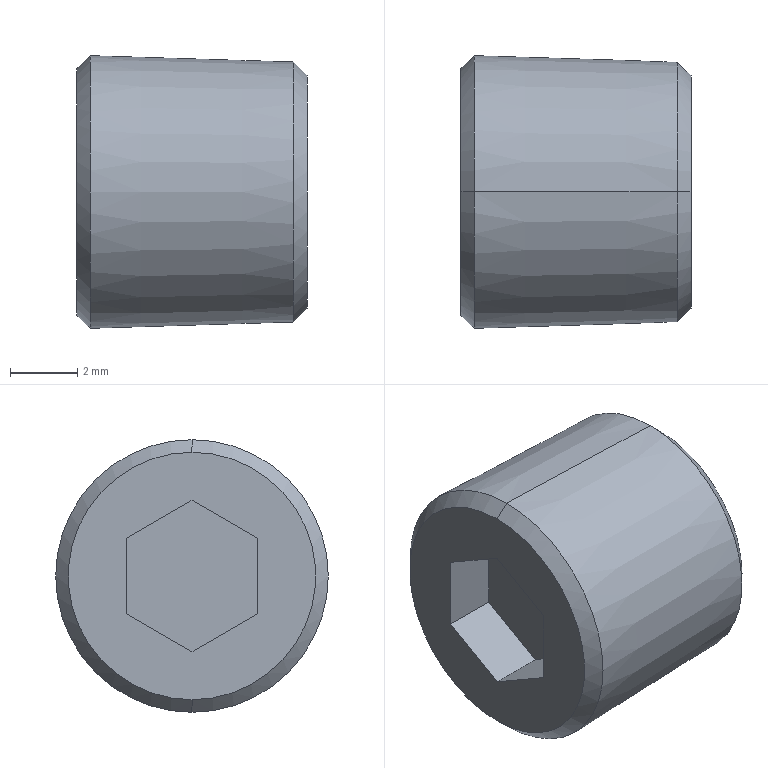Part | STEP file | AC10B-M5_AC3011A Plug(00) | 1 solid | 15 faces | box 6.85 x 8.115 x 8.115 mm | volume 313.171 mm3 | plane 9 | cone 6
STEP:
#1=CARTESIAN_POINT('',(0.,0.,0.));
#2=DIRECTION('',(0.,0.,1.));
#3=DIRECTION('',(1.,0.,0.));
#4=AXIS2_PLACEMENT_3D('',#1,#2,#3);
#5=CARTESIAN_POINT('',(0.,0.,3.682));
#6=VERTEX_POINT('',#5);
#7=CARTESIAN_POINT('',(0.,0.,-3.682));
#8=VERTEX_POINT('',#7);
#9=CARTESIAN_POINT('',(0.,0.,0.));
#10=DIRECTION('',(-1.,0.,0.));
#11=DIRECTION('',(0.,0.,-1.));
#12=AXIS2_PLACEMENT_3D('',#9,#10,#11);
#13=CIRCLE('',#12,3.682);
#14=CARTESIAN_POINT('',(0.,0.,0.));
#15=DIRECTION('',(1.,0.,0.));
#16=DIRECTION('',(0.,0.,-1.));
#17=AXIS2_PLACEMENT_3D('',#14,#15,#16);
#18=CONICAL_SURFACE('',#17,3.682,0.7543);
#19=CARTESIAN_POINT('',(6.283,0.));
#20=DIRECTION('',(-1.,0.));
#21=VECTOR('',#20,1.);
#22=LINE('',#19,#21);
#23=(GEOMETRIC_REPRESENTATION_CONTEXT(2)PARAMETRIC_REPRESENTATION_CONTEXT()REPRESENTATION_CONTEXT('',''));
#24=DEFINITIONAL_REPRESENTATION('',(#22),#23);
#25=PCURVE('',#18,#24);
#26=CARTESIAN_POINT('',(0.,0.,0.));
#27=DIRECTION('',(1.,0.,0.));
#28=DIRECTION('',(0.,0.,-1.));
#29=AXIS2_PLACEMENT_3D('',#26,#27,#28);
#30=PLANE('',#29);
#31=CARTESIAN_POINT('',(3.682,0.));
#32=CARTESIAN_POINT('',(3.682,-6.377));
#33=CARTESIAN_POINT('',(-1.841,-3.188));
#34=CARTESIAN_POINT('',(-7.363,0.));
#35=CARTESIAN_POINT('',(-1.841,3.188));
#36=CARTESIAN_POINT('',(3.682,6.377));
#37=CARTESIAN_POINT('',(3.682,0.));
#38=(BOUNDED_CURVE()B_SPLINE_CURVE(2,(#31,#32,#33,#34,#35,#36,#37),.UNSPECIFIED.,.T.,.F.)B_SPLINE_CURVE_WITH_KNOTS((1,2,2,2,2,1),(-2.094,0.,2.094,4.189,6.283,8.378),.UNSPECIFIED.)CURVE()GEOMETRIC_REPRESENTATION_ITEM()RATIONAL_B_SPLINE_CURVE((1.,0.5,1.,0.5,1.,0.5,1.))REPRESENTATION_ITEM(''));
#39=(GEOMETRIC_REPRESENTATION_CONTEXT(2)PARAMETRIC_REPRESENTATION_CONTEXT()REPRESENTATION_CONTEXT('',''));
#40=DEFINITIONAL_REPRESENTATION('',(#38),#39);
#41=PCURVE('',#30,#40);
#42=SURFACE_CURVE('',#13,(#25,#41),.PCURVE_S1.);
#43=EDGE_CURVE('',#6,#8,#42,.T.);
#44=ORIENTED_EDGE('',*,*,#43,.F.);
#45=CARTESIAN_POINT('',(0.3998,0.,4.057));
#46=VERTEX_POINT('',#45);
#47=CARTESIAN_POINT('',(0.,0.,3.682));
#48=DIRECTION('',(0.7288,0.,0.6848));
#49=VECTOR('',#48,1.);
#50=LINE('',#47,#49);
#51=CARTESIAN_POINT('',(3.142,0.));
#52=DIRECTION('',(0.,1.));
#53=VECTOR('',#52,1.);
#54=LINE('',#51,#53);
#55=(GEOMETRIC_REPRESENTATION_CONTEXT(2)PARAMETRIC_REPRESENTATION_CONTEXT()REPRESENTATION_CONTEXT('',''));
#56=DEFINITIONAL_REPRESENTATION('',(#54),#55);
#57=PCURVE('',#18,#56);
#58=CARTESIAN_POINT('',(0.,0.,0.));
#59=DIRECTION('',(1.,0.,0.));
#60=DIRECTION('',(0.,0.,-1.));
#61=AXIS2_PLACEMENT_3D('',#58,#59,#60);
#62=CONICAL_SURFACE('',#61,3.682,0.7543);
#63=CARTESIAN_POINT('',(3.142,0.));
#64=DIRECTION('',(0.,1.));
#65=VECTOR('',#64,1.);
#66=LINE('',#63,#65);
#67=(GEOMETRIC_REPRESENTATION_CONTEXT(2)PARAMETRIC_REPRESENTATION_CONTEXT()REPRESENTATION_CONTEXT('',''));
#68=DEFINITIONAL_REPRESENTATION('',(#66),#67);
#69=PCURVE('',#62,#68);
#70=SURFACE_CURVE('',#50,(#57,#69),.PCURVE_S1.);
#71=EDGE_CURVE('',#6,#46,#70,.T.);
#72=ORIENTED_EDGE('',*,*,#71,.T.);
#73=CARTESIAN_POINT('',(0.3998,0.,-4.057));
#74=VERTEX_POINT('',#73);
#75=CARTESIAN_POINT('',(0.3998,0.,0.));
#76=DIRECTION('',(1.,0.,0.));
#77=DIRECTION('',(0.,0.,-1.));
#78=AXIS2_PLACEMENT_3D('',#75,#76,#77);
#79=CIRCLE('',#78,4.057);
#80=CARTESIAN_POINT('',(0.,0.3998));
#81=DIRECTION('',(1.,0.));
#82=VECTOR('',#81,1.);
#83=LINE('',#80,#82);
#84=(GEOMETRIC_REPRESENTATION_CONTEXT(2)PARAMETRIC_REPRESENTATION_CONTEXT()REPRESENTATION_CONTEXT('',''));
#85=DEFINITIONAL_REPRESENTATION('',(#83),#84);
#86=PCURVE('',#18,#85);
#87=CARTESIAN_POINT('',(6.85,0.,0.));
#88=DIRECTION('',(-1.,0.,0.));
#89=DIRECTION('',(0.,0.,1.));
#90=AXIS2_PLACEMENT_3D('',#87,#88,#89);
#91=CONICAL_SURFACE('',#90,3.857,0.03112);
#92=CARTESIAN_POINT('',(3.142,6.45));
#93=DIRECTION('',(-1.,0.));
#94=VECTOR('',#93,1.);
#95=LINE('',#92,#94);
#96=(GEOMETRIC_REPRESENTATION_CONTEXT(2)PARAMETRIC_REPRESENTATION_CONTEXT()REPRESENTATION_CONTEXT('',''));
#97=DEFINITIONAL_REPRESENTATION('',(#95),#96);
#98=PCURVE('',#91,#97);
#99=SURFACE_CURVE('',#79,(#86,#98),.PCURVE_S1.);
#100=EDGE_CURVE('',#74,#46,#99,.T.);
#101=ORIENTED_EDGE('',*,*,#100,.F.);
#102=CARTESIAN_POINT('',(0.,0.,-3.682));
#103=DIRECTION('',(0.7288,0.,-0.6848));
#104=VECTOR('',#103,1.);
#105=LINE('',#102,#104);
#106=CARTESIAN_POINT('',(0.,0.));
#107=DIRECTION('',(0.,1.));
#108=VECTOR('',#107,1.);
#109=LINE('',#106,#108);
#110=(GEOMETRIC_REPRESENTATION_CONTEXT(2)PARAMETRIC_REPRESENTATION_CONTEXT()REPRESENTATION_CONTEXT('',''));
#111=DEFINITIONAL_REPRESENTATION('',(#109),#110);
#112=PCURVE('',#18,#111);
#113=CARTESIAN_POINT('',(6.283,0.));
#114=DIRECTION('',(0.,1.));
#115=VECTOR('',#114,1.);
#116=LINE('',#113,#115);
#117=(GEOMETRIC_REPRESENTATION_CONTEXT(2)PARAMETRIC_REPRESENTATION_CONTEXT()REPRESENTATION_CONTEXT('',''));
#118=DEFINITIONAL_REPRESENTATION('',(#116),#117);
#119=PCURVE('',#62,#118);
#120=SURFACE_CURVE('',#105,(#112,#119),.PCURVE_S1.);
#121=EDGE_CURVE('',#8,#74,#120,.T.);
#122=ORIENTED_EDGE('',*,*,#121,.F.);
#123=EDGE_LOOP('',(#44,#72,#101,#122));
#124=FACE_BOUND('',#123,.T.);
#125=ADVANCED_FACE('',(#124),#18,.T.);
#126=CARTESIAN_POINT('',(6.85,0.,-3.457));
#127=VERTEX_POINT('',#126);
#128=CARTESIAN_POINT('',(6.85,0.,3.457));
#129=VERTEX_POINT('',#128);
#130=CARTESIAN_POINT('',(6.85,0.,0.));
#131=DIRECTION('',(1.,0.,0.));
#132=DIRECTION('',(0.,0.,1.));
#133=AXIS2_PLACEMENT_3D('',#130,#131,#132);
#134=CIRCLE('',#133,3.457);
#135=CARTESIAN_POINT('',(6.437,0.,0.));
#136=DIRECTION('',(-1.,0.,0.));
#137=DIRECTION('',(0.,0.,1.));
#138=AXIS2_PLACEMENT_3D('',#135,#136,#137);
#139=CONICAL_SURFACE('',#138,3.869,0.7854);
#140=CARTESIAN_POINT('',(6.283,-0.4129));
#141=DIRECTION('',(-1.,0.));
#142=VECTOR('',#141,1.);
#143=LINE('',#140,#142);
#144=(GEOMETRIC_REPRESENTATION_CONTEXT(2)PARAMETRIC_REPRESENTATION_CONTEXT()REPRESENTATION_CONTEXT('',''));
#145=DEFINITIONAL_REPRESENTATION('',(#143),#144);
#146=PCURVE('',#139,#145);
#147=CARTESIAN_POINT('',(6.85,3.857,0.));
#148=DIRECTION('',(-1.,0.,0.));
#149=DIRECTION('',(0.,0.,1.));
#150=AXIS2_PLACEMENT_3D('',#147,#148,#149);
#151=PLANE('',#150);
#152=CARTESIAN_POINT('',(3.457,-3.857));
#153=CARTESIAN_POINT('',(3.457,-9.844));
#154=CARTESIAN_POINT('',(-1.728,-6.85));
#155=CARTESIAN_POINT('',(-6.913,-3.857));
#156=CARTESIAN_POINT('',(-1.728,-0.8631));
#157=CARTESIAN_POINT('',(3.457,2.13));
#158=CARTESIAN_POINT('',(3.457,-3.857));
#159=(BOUNDED_CURVE()B_SPLINE_CURVE(2,(#152,#153,#154,#155,#156,#157,#158),.UNSPECIFIED.,.T.,.F.)B_SPLINE_CURVE_WITH_KNOTS((1,2,2,2,2,1),(-2.094,0.,2.094,4.189,6.283,8.378),.UNSPECIFIED.)CURVE()GEOMETRIC_REPRESENTATION_ITEM()RATIONAL_B_SPLINE_CURVE((1.,0.5,1.,0.5,1.,0.5,1.))REPRESENTATION_ITEM(''));
#160=(GEOMETRIC_REPRESENTATION_CONTEXT(2)PARAMETRIC_REPRESENTATION_CONTEXT()REPRESENTATION_CONTEXT('',''));
#161=DEFINITIONAL_REPRESENTATION('',(#159),#160);
#162=PCURVE('',#151,#161);
#163=SURFACE_CURVE('',#134,(#146,#162),.PCURVE_S1.);
#164=EDGE_CURVE('',#127,#129,#163,.T.);
#165=ORIENTED_EDGE('',*,*,#164,.F.);
#166=CARTESIAN_POINT('',(6.437,0.,-3.869));
#167=VERTEX_POINT('',#166);
#168=CARTESIAN_POINT('',(6.437,0.,-3.869));
#169=DIRECTION('',(-0.7071,0.,-0.7071));
#170=VECTOR('',#169,1.);
#171=LINE('',#168,#170);
#172=CARTESIAN_POINT('',(3.142,0.));
#173=DIRECTION('',(0.,1.));
#174=VECTOR('',#173,1.);
#175=LINE('',#172,#174);
#176=(GEOMETRIC_REPRESENTATION_CONTEXT(2)PARAMETRIC_REPRESENTATION_CONTEXT()REPRESENTATION_CONTEXT('',''));
#177=DEFINITIONAL_REPRESENTATION('',(#175),#176);
#178=PCURVE('',#139,#177);
#179=CARTESIAN_POINT('',(6.437,0.,0.));
#180=DIRECTION('',(-1.,0.,0.));
#181=DIRECTION('',(0.,0.,1.));
#182=AXIS2_PLACEMENT_3D('',#179,#180,#181);
#183=CONICAL_SURFACE('',#182,3.869,0.7854);
#184=CARTESIAN_POINT('',(3.142,0.));
#185=DIRECTION('',(0.,1.));
#186=VECTOR('',#185,1.);
#187=LINE('',#184,#186);
#188=(GEOMETRIC_REPRESENTATION_CONTEXT(2)PARAMETRIC_REPRESENTATION_CONTEXT()REPRESENTATION_CONTEXT('',''));
#189=DEFINITIONAL_REPRESENTATION('',(#187),#188);
#190=PCURVE('',#183,#189);
#191=SURFACE_CURVE('',#171,(#178,#190),.PCURVE_S1.);
#192=EDGE_CURVE('',#127,#167,#191,.T.);
#193=ORIENTED_EDGE('',*,*,#192,.T.);
#194=CARTESIAN_POINT('',(6.437,0.,3.869));
#195=VERTEX_POINT('',#194);
#196=CARTESIAN_POINT('',(6.437,0.,0.));
#197=DIRECTION('',(-1.,0.,0.));
#198=DIRECTION('',(0.,0.,-1.));
#199=AXIS2_PLACEMENT_3D('',#196,#197,#198);
#200=CIRCLE('',#199,3.869);
#201=CARTESIAN_POINT('',(-3.142,0.));
#202=DIRECTION('',(1.,0.));
#203=VECTOR('',#202,1.);
#204=LINE('',#201,#203);
#205=(GEOMETRIC_REPRESENTATION_CONTEXT(2)PARAMETRIC_REPRESENTATION_CONTEXT()REPRESENTATION_CONTEXT('',''));
#206=DEFINITIONAL_REPRESENTATION('',(#204),#205);
#207=PCURVE('',#139,#206);
#208=CARTESIAN_POINT('',(-3.142,0.4129));
#209=DIRECTION('',(1.,0.));
#210=VECTOR('',#209,1.);
#211=LINE('',#208,#210);
#212=(GEOMETRIC_REPRESENTATION_CONTEXT(2)PARAMETRIC_REPRESENTATION_CONTEXT()REPRESENTATION_CONTEXT('',''));
#213=DEFINITIONAL_REPRESENTATION('',(#211),#212);
#214=PCURVE('',#91,#213);
#215=SURFACE_CURVE('',#200,(#207,#214),.PCURVE_S1.);
#216=EDGE_CURVE('',#195,#167,#215,.T.);
#217=ORIENTED_EDGE('',*,*,#216,.F.);
#218=CARTESIAN_POINT('',(6.437,0.,3.869));
#219=DIRECTION('',(-0.7071,0.,0.7071));
#220=VECTOR('',#219,1.);
#221=LINE('',#218,#220);
#222=CARTESIAN_POINT('',(0.,0.));
#223=DIRECTION('',(0.,1.));
#224=VECTOR('',#223,1.);
#225=LINE('',#222,#224);
#226=(GEOMETRIC_REPRESENTATION_CONTEXT(2)PARAMETRIC_REPRESENTATION_CONTEXT()REPRESENTATION_CONTEXT('',''));
#227=DEFINITIONAL_REPRESENTATION('',(#225),#226);
#228=PCURVE('',#139,#227);
#229=CARTESIAN_POINT('',(6.283,0.));
#230=DIRECTION('',(0.,1.));
#231=VECTOR('',#230,1.);
#232=LINE('',#229,#231);
#233=(GEOMETRIC_REPRESENTATION_CONTEXT(2)PARAMETRIC_REPRESENTATION_CONTEXT()REPRESENTATION_CONTEXT('',''));
#234=DEFINITIONAL_REPRESENTATION('',(#232),#233);
#235=PCURVE('',#183,#234);
#236=SURFACE_CURVE('',#221,(#228,#235),.PCURVE_S1.);
#237=EDGE_CURVE('',#129,#195,#236,.T.);
#238=ORIENTED_EDGE('',*,*,#237,.F.);
#239=EDGE_LOOP('',(#165,#193,#217,#238));
#240=FACE_BOUND('',#239,.T.);
#241=ADVANCED_FACE('',(#240),#139,.T.);
#242=ORIENTED_EDGE('',*,*,#216,.T.);
#243=CARTESIAN_POINT('',(6.85,0.,-3.857));
#244=DIRECTION('',(-0.9995,0.,-0.03111));
#245=VECTOR('',#244,1.);
#246=LINE('',#243,#245);
#247=CARTESIAN_POINT('',(3.142,0.));
#248=DIRECTION('',(0.,1.));
#249=VECTOR('',#248,1.);
#250=LINE('',#247,#249);
#251=(GEOMETRIC_REPRESENTATION_CONTEXT(2)PARAMETRIC_REPRESENTATION_CONTEXT()REPRESENTATION_CONTEXT('',''));
#252=DEFINITIONAL_REPRESENTATION('',(#250),#251);
#253=PCURVE('',#91,#252);
#254=CARTESIAN_POINT('',(6.85,0.,0.));
#255=DIRECTION('',(-1.,0.,0.));
#256=DIRECTION('',(0.,0.,1.));
#257=AXIS2_PLACEMENT_3D('',#254,#255,#256);
#258=CONICAL_SURFACE('',#257,3.857,0.03112);
#259=CARTESIAN_POINT('',(3.142,0.));
#260=DIRECTION('',(0.,1.));
#261=VECTOR('',#260,1.);
#262=LINE('',#259,#261);
#263=(GEOMETRIC_REPRESENTATION_CONTEXT(2)PARAMETRIC_REPRESENTATION_CONTEXT()REPRESENTATION_CONTEXT('',''));
#264=DEFINITIONAL_REPRESENTATION('',(#262),#263);
#265=PCURVE('',#258,#264);
#266=SURFACE_CURVE('',#246,(#253,#265),.PCURVE_S1.);
#267=EDGE_CURVE('',#167,#74,#266,.T.);
#268=ORIENTED_EDGE('',*,*,#267,.T.);
#269=ORIENTED_EDGE('',*,*,#100,.T.);
#270=CARTESIAN_POINT('',(6.85,0.,3.857));
#271=DIRECTION('',(-0.9995,0.,0.03111));
#272=VECTOR('',#271,1.);
#273=LINE('',#270,#272);
#274=CARTESIAN_POINT('',(0.,0.));
#275=DIRECTION('',(0.,1.));
#276=VECTOR('',#275,1.);
#277=LINE('',#274,#276);
#278=(GEOMETRIC_REPRESENTATION_CONTEXT(2)PARAMETRIC_REPRESENTATION_CONTEXT()REPRESENTATION_CONTEXT('',''));
#279=DEFINITIONAL_REPRESENTATION('',(#277),#278);
#280=PCURVE('',#91,#279);
#281=CARTESIAN_POINT('',(6.283,0.));
#282=DIRECTION('',(0.,1.));
#283=VECTOR('',#282,1.);
#284=LINE('',#281,#283);
#285=(GEOMETRIC_REPRESENTATION_CONTEXT(2)PARAMETRIC_REPRESENTATION_CONTEXT()REPRESENTATION_CONTEXT('',''));
#286=DEFINITIONAL_REPRESENTATION('',(#284),#285);
#287=PCURVE('',#258,#286);
#288=SURFACE_CURVE('',#273,(#280,#287),.PCURVE_S1.);
#289=EDGE_CURVE('',#195,#46,#288,.T.);
#290=ORIENTED_EDGE('',*,*,#289,.F.);
#291=EDGE_LOOP('',(#242,#268,#269,#290));
#292=FACE_BOUND('',#291,.T.);
#293=ADVANCED_FACE('',(#292),#91,.T.);
#294=CARTESIAN_POINT('',(0.,0.,2.252));
#295=VERTEX_POINT('',#294);
#296=CARTESIAN_POINT('',(0.,1.95,1.126));
#297=VERTEX_POINT('',#296);
#298=CARTESIAN_POINT('',(0.,0.,2.252));
#299=DIRECTION('',(0.,0.866,-0.5));
#300=VECTOR('',#299,1.);
#301=LINE('',#298,#300);
#302=CARTESIAN_POINT('',(-2.252,0.));
#303=DIRECTION('',(0.5,0.866));
#304=VECTOR('',#303,1.);
#305=LINE('',#302,#304);
#306=(GEOMETRIC_REPRESENTATION_CONTEXT(2)PARAMETRIC_REPRESENTATION_CONTEXT()REPRESENTATION_CONTEXT('',''));
#307=DEFINITIONAL_REPRESENTATION('',(#305),#306);
#308=PCURVE('',#30,#307);
#309=CARTESIAN_POINT('',(1.6,0.,2.252));
#310=DIRECTION('',(0.,0.5,0.866));
#311=DIRECTION('',(0.,-0.866,0.5));
#312=AXIS2_PLACEMENT_3D('',#309,#310,#311);
#313=PLANE('',#312);
#314=CARTESIAN_POINT('',(0.,-1.6));
#315=DIRECTION('',(-1.,0.));
#316=VECTOR('',#315,1.);
#317=LINE('',#314,#316);
#318=(GEOMETRIC_REPRESENTATION_CONTEXT(2)PARAMETRIC_REPRESENTATION_CONTEXT()REPRESENTATION_CONTEXT('',''));
#319=DEFINITIONAL_REPRESENTATION('',(#317),#318);
#320=PCURVE('',#313,#319);
#321=SURFACE_CURVE('',#301,(#308,#320),.PCURVE_S1.);
#322=EDGE_CURVE('',#295,#297,#321,.T.);
#323=ORIENTED_EDGE('',*,*,#322,.F.);
#324=CARTESIAN_POINT('',(0.,-1.95,1.126));
#325=VERTEX_POINT('',#324);
#326=CARTESIAN_POINT('',(0.,-1.95,1.126));
#327=DIRECTION('',(0.,0.866,0.5));
#328=VECTOR('',#327,1.);
#329=LINE('',#326,#328);
#330=CARTESIAN_POINT('',(-1.126,-1.95));
#331=DIRECTION('',(-0.5,0.866));
#332=VECTOR('',#331,1.);
#333=LINE('',#330,#332);
#334=(GEOMETRIC_REPRESENTATION_CONTEXT(2)PARAMETRIC_REPRESENTATION_CONTEXT()REPRESENTATION_CONTEXT('',''));
#335=DEFINITIONAL_REPRESENTATION('',(#333),#334);
#336=PCURVE('',#30,#335);
#337=CARTESIAN_POINT('',(1.6,-1.95,1.126));
#338=DIRECTION('',(0.,-0.5,0.866));
#339=DIRECTION('',(0.,-0.866,-0.5));
#340=AXIS2_PLACEMENT_3D('',#337,#338,#339);
#341=PLANE('',#340);
#342=CARTESIAN_POINT('',(0.,-1.6));
#343=DIRECTION('',(-1.,0.));
#344=VECTOR('',#343,1.);
#345=LINE('',#342,#344);
#346=(GEOMETRIC_REPRESENTATION_CONTEXT(2)PARAMETRIC_REPRESENTATION_CONTEXT()REPRESENTATION_CONTEXT('',''));
#347=DEFINITIONAL_REPRESENTATION('',(#345),#346);
#348=PCURVE('',#341,#347);
#349=SURFACE_CURVE('',#329,(#336,#348),.PCURVE_S1.);
#350=EDGE_CURVE('',#325,#295,#349,.T.);
#351=ORIENTED_EDGE('',*,*,#350,.F.);
#352=CARTESIAN_POINT('',(0.,-1.95,-1.126));
#353=VERTEX_POINT('',#352);
#354=CARTESIAN_POINT('',(0.,-1.95,-1.126));
#355=DIRECTION('',(0.,0.,1.));
#356=VECTOR('',#355,1.);
#357=LINE('',#354,#356);
#358=CARTESIAN_POINT('',(1.126,-1.95));
#359=DIRECTION('',(-1.,0.));
#360=VECTOR('',#359,1.);
#361=LINE('',#358,#360);
#362=(GEOMETRIC_REPRESENTATION_CONTEXT(2)PARAMETRIC_REPRESENTATION_CONTEXT()REPRESENTATION_CONTEXT('',''));
#363=DEFINITIONAL_REPRESENTATION('',(#361),#362);
#364=PCURVE('',#30,#363);
#365=CARTESIAN_POINT('',(1.6,-1.95,-1.126));
#366=DIRECTION('',(0.,-1.,0.));
#367=DIRECTION('',(0.,0.,-1.));
#368=AXIS2_PLACEMENT_3D('',#365,#366,#367);
#369=PLANE('',#368);
#370=CARTESIAN_POINT('',(0.,-1.6));
#371=DIRECTION('',(-1.,0.));
#372=VECTOR('',#371,1.);
#373=LINE('',#370,#372);
#374=(GEOMETRIC_REPRESENTATION_CONTEXT(2)PARAMETRIC_REPRESENTATION_CONTEXT()REPRESENTATION_CONTEXT('',''));
#375=DEFINITIONAL_REPRESENTATION('',(#373),#374);
#376=PCURVE('',#369,#375);
#377=SURFACE_CURVE('',#357,(#364,#376),.PCURVE_S1.);
#378=EDGE_CURVE('',#353,#325,#377,.T.);
#379=ORIENTED_EDGE('',*,*,#378,.F.);
#380=CARTESIAN_POINT('',(0.,0.,-2.252));
#381=VERTEX_POINT('',#380);
#382=CARTESIAN_POINT('',(0.,0.,-2.252));
#383=DIRECTION('',(0.,-0.866,0.5));
#384=VECTOR('',#383,1.);
#385=LINE('',#382,#384);
#386=CARTESIAN_POINT('',(2.252,0.));
#387=DIRECTION('',(-0.5,-0.866));
#388=VECTOR('',#387,1.);
#389=LINE('',#386,#388);
#390=(GEOMETRIC_REPRESENTATION_CONTEXT(2)PARAMETRIC_REPRESENTATION_CONTEXT()REPRESENTATION_CONTEXT('',''));
#391=DEFINITIONAL_REPRESENTATION('',(#389),#390);
#392=PCURVE('',#30,#391);
#393=CARTESIAN_POINT('',(1.6,0.,-2.252));
#394=DIRECTION('',(0.,-0.5,-0.866));
#395=DIRECTION('',(0.,0.866,-0.5));
#396=AXIS2_PLACEMENT_3D('',#393,#394,#395);
#397=PLANE('',#396);
#398=CARTESIAN_POINT('',(0.,-1.6));
#399=DIRECTION('',(-1.,0.));
#400=VECTOR('',#399,1.);
#401=LINE('',#398,#400);
#402=(GEOMETRIC_REPRESENTATION_CONTEXT(2)PARAMETRIC_REPRESENTATION_CONTEXT()REPRESENTATION_CONTEXT('',''));
#403=DEFINITIONAL_REPRESENTATION('',(#401),#402);
#404=PCURVE('',#397,#403);
#405=SURFACE_CURVE('',#385,(#392,#404),.PCURVE_S1.);
#406=EDGE_CURVE('',#381,#353,#405,.T.);
#407=ORIENTED_EDGE('',*,*,#406,.F.);
#408=CARTESIAN_POINT('',(0.,1.95,-1.126));
#409=VERTEX_POINT('',#408);
#410=CARTESIAN_POINT('',(0.,1.95,-1.126));
#411=DIRECTION('',(0.,-0.866,-0.5));
#412=VECTOR('',#411,1.);
#413=LINE('',#410,#412);
#414=CARTESIAN_POINT('',(1.126,1.95));
#415=DIRECTION('',(0.5,-0.866));
#416=VECTOR('',#415,1.);
#417=LINE('',#414,#416);
#418=(GEOMETRIC_REPRESENTATION_CONTEXT(2)PARAMETRIC_REPRESENTATION_CONTEXT()REPRESENTATION_CONTEXT('',''));
#419=DEFINITIONAL_REPRESENTATION('',(#417),#418);
#420=PCURVE('',#30,#419);
#421=CARTESIAN_POINT('',(1.6,1.95,-1.126));
#422=DIRECTION('',(0.,0.5,-0.866));
#423=DIRECTION('',(0.,0.866,0.5));
#424=AXIS2_PLACEMENT_3D('',#421,#422,#423);
#425=PLANE('',#424);
#426=CARTESIAN_POINT('',(0.,-1.6));
#427=DIRECTION('',(-1.,0.));
#428=VECTOR('',#427,1.);
#429=LINE('',#426,#428);
#430=(GEOMETRIC_REPRESENTATION_CONTEXT(2)PARAMETRIC_REPRESENTATION_CONTEXT()REPRESENTATION_CONTEXT('',''));
#431=DEFINITIONAL_REPRESENTATION('',(#429),#430);
#432=PCURVE('',#425,#431);
#433=SURFACE_CURVE('',#413,(#420,#432),.PCURVE_S1.);
#434=EDGE_CURVE('',#409,#381,#433,.T.);
#435=ORIENTED_EDGE('',*,*,#434,.F.);
#436=CARTESIAN_POINT('',(0.,1.95,1.126));
#437=DIRECTION('',(0.,0.,-1.));
#438=VECTOR('',#437,1.);
#439=LINE('',#436,#438);
#440=CARTESIAN_POINT('',(-1.126,1.95));
#441=DIRECTION('',(1.,0.));
#442=VECTOR('',#441,1.);
#443=LINE('',#440,#442);
#444=(GEOMETRIC_REPRESENTATION_CONTEXT(2)PARAMETRIC_REPRESENTATION_CONTEXT()REPRESENTATION_CONTEXT('',''));
#445=DEFINITIONAL_REPRESENTATION('',(#443),#444);
#446=PCURVE('',#30,#445);
#447=CARTESIAN_POINT('',(1.6,1.95,1.126));
#448=DIRECTION('',(0.,1.,0.));
#449=DIRECTION('',(0.,0.,1.));
#450=AXIS2_PLACEMENT_3D('',#447,#448,#449);
#451=PLANE('',#450);
#452=CARTESIAN_POINT('',(0.,-1.6));
#453=DIRECTION('',(-1.,0.));
#454=VECTOR('',#453,1.);
#455=LINE('',#452,#454);
#456=(GEOMETRIC_REPRESENTATION_CONTEXT(2)PARAMETRIC_REPRESENTATION_CONTEXT()REPRESENTATION_CONTEXT('',''));
#457=DEFINITIONAL_REPRESENTATION('',(#455),#456);
#458=PCURVE('',#451,#457);
#459=SURFACE_CURVE('',#439,(#446,#458),.PCURVE_S1.);
#460=EDGE_CURVE('',#297,#409,#459,.T.);
#461=ORIENTED_EDGE('',*,*,#460,.F.);
#462=EDGE_LOOP('',(#323,#351,#379,#407,#435,#461));
#463=FACE_BOUND('',#462,.T.);
#464=CARTESIAN_POINT('',(0.,0.,0.));
#465=DIRECTION('',(-1.,0.,0.));
#466=DIRECTION('',(0.,0.,-1.));
#467=AXIS2_PLACEMENT_3D('',#464,#465,#466);
#468=CIRCLE('',#467,3.682);
#469=CARTESIAN_POINT('',(3.682,0.));
#470=CARTESIAN_POINT('',(3.682,-6.377));
#471=CARTESIAN_POINT('',(-1.841,-3.188));
#472=CARTESIAN_POINT('',(-7.363,0.));
#473=CARTESIAN_POINT('',(-1.841,3.188));
#474=CARTESIAN_POINT('',(3.682,6.377));
#475=CARTESIAN_POINT('',(3.682,0.));
#476=(BOUNDED_CURVE()B_SPLINE_CURVE(2,(#469,#470,#471,#472,#473,#474,#475),.UNSPECIFIED.,.T.,.F.)B_SPLINE_CURVE_WITH_KNOTS((1,2,2,2,2,1),(-2.094,0.,2.094,4.189,6.283,8.378),.UNSPECIFIED.)CURVE()GEOMETRIC_REPRESENTATION_ITEM()RATIONAL_B_SPLINE_CURVE((1.,0.5,1.,0.5,1.,0.5,1.))REPRESENTATION_ITEM(''));
#477=(GEOMETRIC_REPRESENTATION_CONTEXT(2)PARAMETRIC_REPRESENTATION_CONTEXT()REPRESENTATION_CONTEXT('',''));
#478=DEFINITIONAL_REPRESENTATION('',(#476),#477);
#479=PCURVE('',#30,#478);
#480=CARTESIAN_POINT('',(6.283,0.));
#481=DIRECTION('',(-1.,0.));
#482=VECTOR('',#481,1.);
#483=LINE('',#480,#482);
#484=(GEOMETRIC_REPRESENTATION_CONTEXT(2)PARAMETRIC_REPRESENTATION_CONTEXT()REPRESENTATION_CONTEXT('',''));
#485=DEFINITIONAL_REPRESENTATION('',(#483),#484);
#486=PCURVE('',#62,#485);
#487=SURFACE_CURVE('',#468,(#479,#486),.PCURVE_S1.);
#488=EDGE_CURVE('',#8,#6,#487,.T.);
#489=ORIENTED_EDGE('',*,*,#488,.T.);
#490=ORIENTED_EDGE('',*,*,#43,.T.);
#491=EDGE_LOOP('',(#489,#490));
#492=FACE_BOUND('',#491,.T.);
#493=ADVANCED_FACE('',(#463,#492),#30,.F.);
#494=ORIENTED_EDGE('',*,*,#267,.F.);
#495=CARTESIAN_POINT('',(6.437,0.,0.));
#496=DIRECTION('',(-1.,0.,0.));
#497=DIRECTION('',(0.,0.,-1.));
#498=AXIS2_PLACEMENT_3D('',#495,#496,#497);
#499=CIRCLE('',#498,3.869);
#500=CARTESIAN_POINT('',(3.142,0.4129));
#501=DIRECTION('',(1.,0.));
#502=VECTOR('',#501,1.);
#503=LINE('',#500,#502);
#504=(GEOMETRIC_REPRESENTATION_CONTEXT(2)PARAMETRIC_REPRESENTATION_CONTEXT()REPRESENTATION_CONTEXT('',''));
#505=DEFINITIONAL_REPRESENTATION('',(#503),#504);
#506=PCURVE('',#258,#505);
#507=CARTESIAN_POINT('',(3.142,0.));
#508=DIRECTION('',(1.,0.));
#509=VECTOR('',#508,1.);
#510=LINE('',#507,#509);
#511=(GEOMETRIC_REPRESENTATION_CONTEXT(2)PARAMETRIC_REPRESENTATION_CONTEXT()REPRESENTATION_CONTEXT('',''));
#512=DEFINITIONAL_REPRESENTATION('',(#510),#511);
#513=PCURVE('',#183,#512);
#514=SURFACE_CURVE('',#499,(#506,#513),.PCURVE_S1.);
#515=EDGE_CURVE('',#167,#195,#514,.T.);
#516=ORIENTED_EDGE('',*,*,#515,.T.);
#517=ORIENTED_EDGE('',*,*,#289,.T.);
#518=CARTESIAN_POINT('',(0.3998,0.,0.));
#519=DIRECTION('',(1.,0.,0.));
#520=DIRECTION('',(0.,0.,-1.));
#521=AXIS2_PLACEMENT_3D('',#518,#519,#520);
#522=CIRCLE('',#521,4.057);
#523=CARTESIAN_POINT('',(9.425,6.45));
#524=DIRECTION('',(-1.,0.));
#525=VECTOR('',#524,1.);
#526=LINE('',#523,#525);
#527=(GEOMETRIC_REPRESENTATION_CONTEXT(2)PARAMETRIC_REPRESENTATION_CONTEXT()REPRESENTATION_CONTEXT('',''));
#528=DEFINITIONAL_REPRESENTATION('',(#526),#527);
#529=PCURVE('',#258,#528);
#530=CARTESIAN_POINT('',(0.,0.3998));
#531=DIRECTION('',(1.,0.));
#532=VECTOR('',#531,1.);
#533=LINE('',#530,#532);
#534=(GEOMETRIC_REPRESENTATION_CONTEXT(2)PARAMETRIC_REPRESENTATION_CONTEXT()REPRESENTATION_CONTEXT('',''));
#535=DEFINITIONAL_REPRESENTATION('',(#533),#534);
#536=PCURVE('',#62,#535);
#537=SURFACE_CURVE('',#522,(#529,#536),.PCURVE_S1.);
#538=EDGE_CURVE('',#46,#74,#537,.T.);
#539=ORIENTED_EDGE('',*,*,#538,.T.);
#540=EDGE_LOOP('',(#494,#516,#517,#539));
#541=FACE_BOUND('',#540,.T.);
#542=ADVANCED_FACE('',(#541),#258,.T.);
#543=CARTESIAN_POINT('',(6.85,0.,0.));
#544=DIRECTION('',(1.,0.,0.));
#545=DIRECTION('',(0.,0.,1.));
#546=AXIS2_PLACEMENT_3D('',#543,#544,#545);
#547=CIRCLE('',#546,3.457);
#548=CARTESIAN_POINT('',(3.457,-3.857));
#549=CARTESIAN_POINT('',(3.457,-9.844));
#550=CARTESIAN_POINT('',(-1.728,-6.85));
#551=CARTESIAN_POINT('',(-6.913,-3.857));
#552=CARTESIAN_POINT('',(-1.728,-0.8631));
#553=CARTESIAN_POINT('',(3.457,2.13));
#554=CARTESIAN_POINT('',(3.457,-3.857));
#555=(BOUNDED_CURVE()B_SPLINE_CURVE(2,(#548,#549,#550,#551,#552,#553,#554),.UNSPECIFIED.,.T.,.F.)B_SPLINE_CURVE_WITH_KNOTS((1,2,2,2,2,1),(-2.094,0.,2.094,4.189,6.283,8.378),.UNSPECIFIED.)CURVE()GEOMETRIC_REPRESENTATION_ITEM()RATIONAL_B_SPLINE_CURVE((1.,0.5,1.,0.5,1.,0.5,1.))REPRESENTATION_ITEM(''));
#556=(GEOMETRIC_REPRESENTATION_CONTEXT(2)PARAMETRIC_REPRESENTATION_CONTEXT()REPRESENTATION_CONTEXT('',''));
#557=DEFINITIONAL_REPRESENTATION('',(#555),#556);
#558=PCURVE('',#151,#557);
#559=CARTESIAN_POINT('',(6.283,-0.4129));
#560=DIRECTION('',(-1.,0.));
#561=VECTOR('',#560,1.);
#562=LINE('',#559,#561);
#563=(GEOMETRIC_REPRESENTATION_CONTEXT(2)PARAMETRIC_REPRESENTATION_CONTEXT()REPRESENTATION_CONTEXT('',''));
#564=DEFINITIONAL_REPRESENTATION('',(#562),#563);
#565=PCURVE('',#183,#564);
#566=SURFACE_CURVE('',#547,(#558,#565),.PCURVE_S1.);
#567=EDGE_CURVE('',#129,#127,#566,.T.);
#568=ORIENTED_EDGE('',*,*,#567,.T.);
#569=ORIENTED_EDGE('',*,*,#164,.T.);
#570=EDGE_LOOP('',(#568,#569));
#571=FACE_BOUND('',#570,.T.);
#572=ADVANCED_FACE('',(#571),#151,.F.);
#573=ORIENTED_EDGE('',*,*,#192,.F.);
#574=ORIENTED_EDGE('',*,*,#567,.F.);
#575=ORIENTED_EDGE('',*,*,#237,.T.);
#576=ORIENTED_EDGE('',*,*,#515,.F.);
#577=EDGE_LOOP('',(#573,#574,#575,#576));
#578=FACE_BOUND('',#577,.T.);
#579=ADVANCED_FACE('',(#578),#183,.T.);
#580=ORIENTED_EDGE('',*,*,#71,.F.);
#581=ORIENTED_EDGE('',*,*,#488,.F.);
#582=ORIENTED_EDGE('',*,*,#121,.T.);
#583=ORIENTED_EDGE('',*,*,#538,.F.);
#584=EDGE_LOOP('',(#580,#581,#582,#583));
#585=FACE_BOUND('',#584,.T.);
#586=ADVANCED_FACE('',(#585),#62,.T.);
#587=ORIENTED_EDGE('',*,*,#350,.T.);
#588=CARTESIAN_POINT('',(1.6,0.,2.252));
#589=VERTEX_POINT('',#588);
#590=CARTESIAN_POINT('',(1.6,0.,2.252));
#591=DIRECTION('',(-1.,0.,0.));
#592=VECTOR('',#591,1.);
#593=LINE('',#590,#592);
#594=CARTESIAN_POINT('',(-2.252,0.));
#595=DIRECTION('',(0.,-1.));
#596=VECTOR('',#595,1.);
#597=LINE('',#594,#596);
#598=(GEOMETRIC_REPRESENTATION_CONTEXT(2)PARAMETRIC_REPRESENTATION_CONTEXT()REPRESENTATION_CONTEXT('',''));
#599=DEFINITIONAL_REPRESENTATION('',(#597),#598);
#600=PCURVE('',#341,#599);
#601=CARTESIAN_POINT('',(0.,0.));
#602=DIRECTION('',(0.,-1.));
#603=VECTOR('',#602,1.);
#604=LINE('',#601,#603);
#605=(GEOMETRIC_REPRESENTATION_CONTEXT(2)PARAMETRIC_REPRESENTATION_CONTEXT()REPRESENTATION_CONTEXT('',''));
#606=DEFINITIONAL_REPRESENTATION('',(#604),#605);
#607=PCURVE('',#313,#606);
#608=SURFACE_CURVE('',#593,(#600,#607),.PCURVE_S1.);
#609=EDGE_CURVE('',#589,#295,#608,.T.);
#610=ORIENTED_EDGE('',*,*,#609,.F.);
#611=CARTESIAN_POINT('',(1.6,-1.95,1.126));
#612=VERTEX_POINT('',#611);
#613=CARTESIAN_POINT('',(1.6,-1.95,1.126));
#614=DIRECTION('',(0.,0.866,0.5));
#615=VECTOR('',#614,1.);
#616=LINE('',#613,#615);
#617=CARTESIAN_POINT('',(0.,0.));
#618=DIRECTION('',(-1.,0.));
#619=VECTOR('',#618,1.);
#620=LINE('',#617,#619);
#621=(GEOMETRIC_REPRESENTATION_CONTEXT(2)PARAMETRIC_REPRESENTATION_CONTEXT()REPRESENTATION_CONTEXT('',''));
#622=DEFINITIONAL_REPRESENTATION('',(#620),#621);
#623=PCURVE('',#341,#622);
#624=CARTESIAN_POINT('',(1.6,-1.95,1.126));
#625=DIRECTION('',(1.,0.,0.));
#626=DIRECTION('',(0.,0.,-1.));
#627=AXIS2_PLACEMENT_3D('',#624,#625,#626);
#628=PLANE('',#627);
#629=CARTESIAN_POINT('',(0.,0.));
#630=DIRECTION('',(-0.5,0.866));
#631=VECTOR('',#630,1.);
#632=LINE('',#629,#631);
#633=(GEOMETRIC_REPRESENTATION_CONTEXT(2)PARAMETRIC_REPRESENTATION_CONTEXT()REPRESENTATION_CONTEXT('',''));
#634=DEFINITIONAL_REPRESENTATION('',(#632),#633);
#635=PCURVE('',#628,#634);
#636=SURFACE_CURVE('',#616,(#623,#635),.PCURVE_S1.);
#637=EDGE_CURVE('',#612,#589,#636,.T.);
#638=ORIENTED_EDGE('',*,*,#637,.F.);
#639=CARTESIAN_POINT('',(1.6,-1.95,1.126));
#640=DIRECTION('',(-1.,0.,0.));
#641=VECTOR('',#640,1.);
#642=LINE('',#639,#641);
#643=CARTESIAN_POINT('',(0.,0.));
#644=DIRECTION('',(0.,-1.));
#645=VECTOR('',#644,1.);
#646=LINE('',#643,#645);
#647=(GEOMETRIC_REPRESENTATION_CONTEXT(2)PARAMETRIC_REPRESENTATION_CONTEXT()REPRESENTATION_CONTEXT('',''));
#648=DEFINITIONAL_REPRESENTATION('',(#646),#647);
#649=PCURVE('',#341,#648);
#650=CARTESIAN_POINT('',(-2.252,0.));
#651=DIRECTION('',(0.,-1.));
#652=VECTOR('',#651,1.);
#653=LINE('',#650,#652);
#654=(GEOMETRIC_REPRESENTATION_CONTEXT(2)PARAMETRIC_REPRESENTATION_CONTEXT()REPRESENTATION_CONTEXT('',''));
#655=DEFINITIONAL_REPRESENTATION('',(#653),#654);
#656=PCURVE('',#369,#655);
#657=SURFACE_CURVE('',#642,(#649,#656),.PCURVE_S1.);
#658=EDGE_CURVE('',#612,#325,#657,.T.);
#659=ORIENTED_EDGE('',*,*,#658,.T.);
#660=EDGE_LOOP('',(#587,#610,#638,#659));
#661=FACE_BOUND('',#660,.T.);
#662=ADVANCED_FACE('',(#661),#341,.F.);
#663=ORIENTED_EDGE('',*,*,#378,.T.);
#664=ORIENTED_EDGE('',*,*,#658,.F.);
#665=CARTESIAN_POINT('',(1.6,-1.95,-1.126));
#666=VERTEX_POINT('',#665);
#667=CARTESIAN_POINT('',(1.6,-1.95,-1.126));
#668=DIRECTION('',(0.,0.,1.));
#669=VECTOR('',#668,1.);
#670=LINE('',#667,#669);
#671=CARTESIAN_POINT('',(0.,0.));
#672=DIRECTION('',(-1.,0.));
#673=VECTOR('',#672,1.);
#674=LINE('',#671,#673);
#675=(GEOMETRIC_REPRESENTATION_CONTEXT(2)PARAMETRIC_REPRESENTATION_CONTEXT()REPRESENTATION_CONTEXT('',''));
#676=DEFINITIONAL_REPRESENTATION('',(#674),#675);
#677=PCURVE('',#369,#676);
#678=CARTESIAN_POINT('',(2.252,0.));
#679=DIRECTION('',(-1.,0.));
#680=VECTOR('',#679,1.);
#681=LINE('',#678,#680);
#682=(GEOMETRIC_REPRESENTATION_CONTEXT(2)PARAMETRIC_REPRESENTATION_CONTEXT()REPRESENTATION_CONTEXT('',''));
#683=DEFINITIONAL_REPRESENTATION('',(#681),#682);
#684=PCURVE('',#628,#683);
#685=SURFACE_CURVE('',#670,(#677,#684),.PCURVE_S1.);
#686=EDGE_CURVE('',#666,#612,#685,.T.);
#687=ORIENTED_EDGE('',*,*,#686,.F.);
#688=CARTESIAN_POINT('',(1.6,-1.95,-1.126));
#689=DIRECTION('',(-1.,0.,0.));
#690=VECTOR('',#689,1.);
#691=LINE('',#688,#690);
#692=CARTESIAN_POINT('',(0.,0.));
#693=DIRECTION('',(0.,-1.));
#694=VECTOR('',#693,1.);
#695=LINE('',#692,#694);
#696=(GEOMETRIC_REPRESENTATION_CONTEXT(2)PARAMETRIC_REPRESENTATION_CONTEXT()REPRESENTATION_CONTEXT('',''));
#697=DEFINITIONAL_REPRESENTATION('',(#695),#696);
#698=PCURVE('',#369,#697);
#699=CARTESIAN_POINT('',(-2.252,0.));
#700=DIRECTION('',(0.,-1.));
#701=VECTOR('',#700,1.);
#702=LINE('',#699,#701);
#703=(GEOMETRIC_REPRESENTATION_CONTEXT(2)PARAMETRIC_REPRESENTATION_CONTEXT()REPRESENTATION_CONTEXT('',''));
#704=DEFINITIONAL_REPRESENTATION('',(#702),#703);
#705=PCURVE('',#397,#704);
#706=SURFACE_CURVE('',#691,(#698,#705),.PCURVE_S1.);
#707=EDGE_CURVE('',#666,#353,#706,.T.);
#708=ORIENTED_EDGE('',*,*,#707,.T.);
#709=EDGE_LOOP('',(#663,#664,#687,#708));
#710=FACE_BOUND('',#709,.T.);
#711=ADVANCED_FACE('',(#710),#369,.F.);
#712=ORIENTED_EDGE('',*,*,#406,.T.);
#713=ORIENTED_EDGE('',*,*,#707,.F.);
#714=CARTESIAN_POINT('',(1.6,0.,-2.252));
#715=VERTEX_POINT('',#714);
#716=CARTESIAN_POINT('',(1.6,0.,-2.252));
#717=DIRECTION('',(0.,-0.866,0.5));
#718=VECTOR('',#717,1.);
#719=LINE('',#716,#718);
#720=CARTESIAN_POINT('',(0.,0.));
#721=DIRECTION('',(-1.,0.));
#722=VECTOR('',#721,1.);
#723=LINE('',#720,#722);
#724=(GEOMETRIC_REPRESENTATION_CONTEXT(2)PARAMETRIC_REPRESENTATION_CONTEXT()REPRESENTATION_CONTEXT('',''));
#725=DEFINITIONAL_REPRESENTATION('',(#723),#724);
#726=PCURVE('',#397,#725);
#727=CARTESIAN_POINT('',(3.377,1.95));
#728=DIRECTION('',(-0.5,-0.866));
#729=VECTOR('',#728,1.);
#730=LINE('',#727,#729);
#731=(GEOMETRIC_REPRESENTATION_CONTEXT(2)PARAMETRIC_REPRESENTATION_CONTEXT()REPRESENTATION_CONTEXT('',''));
#732=DEFINITIONAL_REPRESENTATION('',(#730),#731);
#733=PCURVE('',#628,#732);
#734=SURFACE_CURVE('',#719,(#726,#733),.PCURVE_S1.);
#735=EDGE_CURVE('',#715,#666,#734,.T.);
#736=ORIENTED_EDGE('',*,*,#735,.F.);
#737=CARTESIAN_POINT('',(1.6,0.,-2.252));
#738=DIRECTION('',(-1.,0.,0.));
#739=VECTOR('',#738,1.);
#740=LINE('',#737,#739);
#741=CARTESIAN_POINT('',(0.,0.));
#742=DIRECTION('',(0.,-1.));
#743=VECTOR('',#742,1.);
#744=LINE('',#741,#743);
#745=(GEOMETRIC_REPRESENTATION_CONTEXT(2)PARAMETRIC_REPRESENTATION_CONTEXT()REPRESENTATION_CONTEXT('',''));
#746=DEFINITIONAL_REPRESENTATION('',(#744),#745);
#747=PCURVE('',#397,#746);
#748=CARTESIAN_POINT('',(-2.252,0.));
#749=DIRECTION('',(0.,-1.));
#750=VECTOR('',#749,1.);
#751=LINE('',#748,#750);
#752=(GEOMETRIC_REPRESENTATION_CONTEXT(2)PARAMETRIC_REPRESENTATION_CONTEXT()REPRESENTATION_CONTEXT('',''));
#753=DEFINITIONAL_REPRESENTATION('',(#751),#752);
#754=PCURVE('',#425,#753);
#755=SURFACE_CURVE('',#740,(#747,#754),.PCURVE_S1.);
#756=EDGE_CURVE('',#715,#381,#755,.T.);
#757=ORIENTED_EDGE('',*,*,#756,.T.);
#758=EDGE_LOOP('',(#712,#713,#736,#757));
#759=FACE_BOUND('',#758,.T.);
#760=ADVANCED_FACE('',(#759),#397,.F.);
#761=ORIENTED_EDGE('',*,*,#434,.T.);
#762=ORIENTED_EDGE('',*,*,#756,.F.);
#763=CARTESIAN_POINT('',(1.6,1.95,-1.126));
#764=VERTEX_POINT('',#763);
#765=CARTESIAN_POINT('',(1.6,1.95,-1.126));
#766=DIRECTION('',(0.,-0.866,-0.5));
#767=VECTOR('',#766,1.);
#768=LINE('',#765,#767);
#769=CARTESIAN_POINT('',(0.,0.));
#770=DIRECTION('',(-1.,0.));
#771=VECTOR('',#770,1.);
#772=LINE('',#769,#771);
#773=(GEOMETRIC_REPRESENTATION_CONTEXT(2)PARAMETRIC_REPRESENTATION_CONTEXT()REPRESENTATION_CONTEXT('',''));
#774=DEFINITIONAL_REPRESENTATION('',(#772),#773);
#775=PCURVE('',#425,#774);
#776=CARTESIAN_POINT('',(2.252,3.9));
#777=DIRECTION('',(0.5,-0.866));
#778=VECTOR('',#777,1.);
#779=LINE('',#776,#778);
#780=(GEOMETRIC_REPRESENTATION_CONTEXT(2)PARAMETRIC_REPRESENTATION_CONTEXT()REPRESENTATION_CONTEXT('',''));
#781=DEFINITIONAL_REPRESENTATION('',(#779),#780);
#782=PCURVE('',#628,#781);
#783=SURFACE_CURVE('',#768,(#775,#782),.PCURVE_S1.);
#784=EDGE_CURVE('',#764,#715,#783,.T.);
#785=ORIENTED_EDGE('',*,*,#784,.F.);
#786=CARTESIAN_POINT('',(1.6,1.95,-1.126));
#787=DIRECTION('',(-1.,0.,0.));
#788=VECTOR('',#787,1.);
#789=LINE('',#786,#788);
#790=CARTESIAN_POINT('',(0.,0.));
#791=DIRECTION('',(0.,-1.));
#792=VECTOR('',#791,1.);
#793=LINE('',#790,#792);
#794=(GEOMETRIC_REPRESENTATION_CONTEXT(2)PARAMETRIC_REPRESENTATION_CONTEXT()REPRESENTATION_CONTEXT('',''));
#795=DEFINITIONAL_REPRESENTATION('',(#793),#794);
#796=PCURVE('',#425,#795);
#797=CARTESIAN_POINT('',(-2.252,0.));
#798=DIRECTION('',(0.,-1.));
#799=VECTOR('',#798,1.);
#800=LINE('',#797,#799);
#801=(GEOMETRIC_REPRESENTATION_CONTEXT(2)PARAMETRIC_REPRESENTATION_CONTEXT()REPRESENTATION_CONTEXT('',''));
#802=DEFINITIONAL_REPRESENTATION('',(#800),#801);
#803=PCURVE('',#451,#802);
#804=SURFACE_CURVE('',#789,(#796,#803),.PCURVE_S1.);
#805=EDGE_CURVE('',#764,#409,#804,.T.);
#806=ORIENTED_EDGE('',*,*,#805,.T.);
#807=EDGE_LOOP('',(#761,#762,#785,#806));
#808=FACE_BOUND('',#807,.T.);
#809=ADVANCED_FACE('',(#808),#425,.F.);
#810=ORIENTED_EDGE('',*,*,#460,.T.);
#811=ORIENTED_EDGE('',*,*,#805,.F.);
#812=CARTESIAN_POINT('',(1.6,1.95,1.126));
#813=VERTEX_POINT('',#812);
#814=CARTESIAN_POINT('',(1.6,1.95,1.126));
#815=DIRECTION('',(0.,0.,-1.));
#816=VECTOR('',#815,1.);
#817=LINE('',#814,#816);
#818=CARTESIAN_POINT('',(0.,0.));
#819=DIRECTION('',(-1.,0.));
#820=VECTOR('',#819,1.);
#821=LINE('',#818,#820);
#822=(GEOMETRIC_REPRESENTATION_CONTEXT(2)PARAMETRIC_REPRESENTATION_CONTEXT()REPRESENTATION_CONTEXT('',''));
#823=DEFINITIONAL_REPRESENTATION('',(#821),#822);
#824=PCURVE('',#451,#823);
#825=CARTESIAN_POINT('',(0.,3.9));
#826=DIRECTION('',(1.,0.));
#827=VECTOR('',#826,1.);
#828=LINE('',#825,#827);
#829=(GEOMETRIC_REPRESENTATION_CONTEXT(2)PARAMETRIC_REPRESENTATION_CONTEXT()REPRESENTATION_CONTEXT('',''));
#830=DEFINITIONAL_REPRESENTATION('',(#828),#829);
#831=PCURVE('',#628,#830);
#832=SURFACE_CURVE('',#817,(#824,#831),.PCURVE_S1.);
#833=EDGE_CURVE('',#813,#764,#832,.T.);
#834=ORIENTED_EDGE('',*,*,#833,.F.);
#835=CARTESIAN_POINT('',(1.6,1.95,1.126));
#836=DIRECTION('',(-1.,0.,0.));
#837=VECTOR('',#836,1.);
#838=LINE('',#835,#837);
#839=CARTESIAN_POINT('',(0.,0.));
#840=DIRECTION('',(0.,-1.));
#841=VECTOR('',#840,1.);
#842=LINE('',#839,#841);
#843=(GEOMETRIC_REPRESENTATION_CONTEXT(2)PARAMETRIC_REPRESENTATION_CONTEXT()REPRESENTATION_CONTEXT('',''));
#844=DEFINITIONAL_REPRESENTATION('',(#842),#843);
#845=PCURVE('',#451,#844);
#846=CARTESIAN_POINT('',(-2.252,0.));
#847=DIRECTION('',(0.,-1.));
#848=VECTOR('',#847,1.);
#849=LINE('',#846,#848);
#850=(GEOMETRIC_REPRESENTATION_CONTEXT(2)PARAMETRIC_REPRESENTATION_CONTEXT()REPRESENTATION_CONTEXT('',''));
#851=DEFINITIONAL_REPRESENTATION('',(#849),#850);
#852=PCURVE('',#313,#851);
#853=SURFACE_CURVE('',#838,(#845,#852),.PCURVE_S1.);
#854=EDGE_CURVE('',#813,#297,#853,.T.);
#855=ORIENTED_EDGE('',*,*,#854,.T.);
#856=EDGE_LOOP('',(#810,#811,#834,#855));
#857=FACE_BOUND('',#856,.T.);
#858=ADVANCED_FACE('',(#857),#451,.F.);
#859=ORIENTED_EDGE('',*,*,#322,.T.);
#860=ORIENTED_EDGE('',*,*,#854,.F.);
#861=CARTESIAN_POINT('',(1.6,0.,2.252));
#862=DIRECTION('',(0.,0.866,-0.5));
#863=VECTOR('',#862,1.);
#864=LINE('',#861,#863);
#865=CARTESIAN_POINT('',(0.,0.));
#866=DIRECTION('',(-1.,0.));
#867=VECTOR('',#866,1.);
#868=LINE('',#865,#867);
#869=(GEOMETRIC_REPRESENTATION_CONTEXT(2)PARAMETRIC_REPRESENTATION_CONTEXT()REPRESENTATION_CONTEXT('',''));
#870=DEFINITIONAL_REPRESENTATION('',(#868),#869);
#871=PCURVE('',#313,#870);
#872=CARTESIAN_POINT('',(-1.126,1.95));
#873=DIRECTION('',(0.5,0.866));
#874=VECTOR('',#873,1.);
#875=LINE('',#872,#874);
#876=(GEOMETRIC_REPRESENTATION_CONTEXT(2)PARAMETRIC_REPRESENTATION_CONTEXT()REPRESENTATION_CONTEXT('',''));
#877=DEFINITIONAL_REPRESENTATION('',(#875),#876);
#878=PCURVE('',#628,#877);
#879=SURFACE_CURVE('',#864,(#871,#878),.PCURVE_S1.);
#880=EDGE_CURVE('',#589,#813,#879,.T.);
#881=ORIENTED_EDGE('',*,*,#880,.F.);
#882=ORIENTED_EDGE('',*,*,#609,.T.);
#883=EDGE_LOOP('',(#859,#860,#881,#882));
#884=FACE_BOUND('',#883,.T.);
#885=ADVANCED_FACE('',(#884),#313,.F.);
#886=ORIENTED_EDGE('',*,*,#637,.T.);
#887=ORIENTED_EDGE('',*,*,#880,.T.);
#888=ORIENTED_EDGE('',*,*,#833,.T.);
#889=ORIENTED_EDGE('',*,*,#784,.T.);
#890=ORIENTED_EDGE('',*,*,#735,.T.);
#891=ORIENTED_EDGE('',*,*,#686,.T.);
#892=EDGE_LOOP('',(#886,#887,#888,#889,#890,#891));
#893=FACE_BOUND('',#892,.T.);
#894=ADVANCED_FACE('',(#893),#628,.F.);
#895=CLOSED_SHELL('',(#125,#241,#293,#493,#542,#572,#579,#586,#662,#711,#760,#809,#858,#885,#894));
#896=MANIFOLD_SOLID_BREP('',#895);
#897=(LENGTH_UNIT()NAMED_UNIT(*)SI_UNIT(.MILLI.,.METRE.));
#898=UNCERTAINTY_MEASURE_WITH_UNIT(LENGTH_MEASURE(0.0000001),#897,'','');
#899=(NAMED_UNIT(*)PLANE_ANGLE_UNIT()SI_UNIT($,.RADIAN.));
#900=(NAMED_UNIT(*)SI_UNIT($,.STERADIAN.)SOLID_ANGLE_UNIT());
#901=(GEOMETRIC_REPRESENTATION_CONTEXT(3)GLOBAL_UNCERTAINTY_ASSIGNED_CONTEXT((#898))GLOBAL_UNIT_ASSIGNED_CONTEXT((#897,#899,#900))REPRESENTATION_CONTEXT('',''));
#902=ADVANCED_BREP_SHAPE_REPRESENTATION('',(#4,#896),#901);